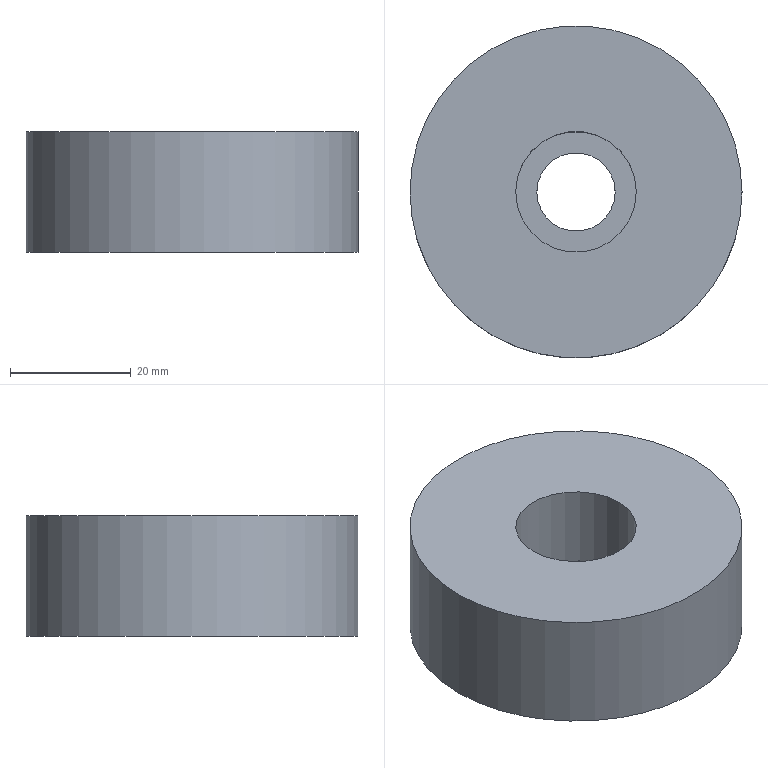Part | NX | features solid 2 | 1 solid | 6 faces | box 55 x 55 x 20 mm | volume 42322 mm3 | cylinder 3 | plane 3 | commonest cylinder face diameters 13 x1 20 x1 55 x1
STEP:
#1=CARTESIAN_POINT('',(512.5,735.,223.2));
#2=VERTEX_POINT('',#1);
#3=CARTESIAN_POINT('',(540.,735.,223.2));
#4=DIRECTION('',(0.,0.,-1.));
#5=DIRECTION('',(-1.,0.,0.));
#6=AXIS2_PLACEMENT_3D('',#3,#4,#5);
#7=CIRCLE('',#6,27.5);
#8=EDGE_CURVE('',#2,#2,#7,.T.);
#9=ORIENTED_EDGE('',*,*,#8,.T.);
#10=EDGE_LOOP('',(#9));
#11=FACE_BOUND('',#10,.T.);
#12=CARTESIAN_POINT('',(512.5,735.,203.2));
#13=VERTEX_POINT('',#12);
#14=CARTESIAN_POINT('',(540.,735.,203.2));
#15=DIRECTION('',(0.,0.,-1.));
#16=DIRECTION('',(-1.,0.,0.));
#17=AXIS2_PLACEMENT_3D('',#14,#15,#16);
#18=CIRCLE('',#17,27.5);
#19=EDGE_CURVE('',#13,#13,#18,.T.);
#20=ORIENTED_EDGE('',*,*,#19,.F.);
#21=EDGE_LOOP('',(#20));
#22=FACE_BOUND('',#21,.T.);
#23=CARTESIAN_POINT('',(540.,735.,223.2));
#24=DIRECTION('',(0.,0.,-1.));
#25=DIRECTION('',(1.,0.,0.));
#26=AXIS2_PLACEMENT_3D('',#23,#24,#25);
#27=CYLINDRICAL_SURFACE('',#26,27.5);
#28=ADVANCED_FACE('',(#11,#22),#27,.T.);
#29=CARTESIAN_POINT('',(550.,735.,223.2));
#30=VERTEX_POINT('',#29);
#31=CARTESIAN_POINT('',(540.,735.,223.2));
#32=DIRECTION('',(0.,0.,1.));
#33=DIRECTION('',(1.,0.,0.));
#34=AXIS2_PLACEMENT_3D('',#31,#32,#33);
#35=CIRCLE('',#34,10.);
#36=EDGE_CURVE('',#30,#30,#35,.T.);
#37=ORIENTED_EDGE('',*,*,#36,.F.);
#38=EDGE_LOOP('',(#37));
#39=FACE_BOUND('',#38,.T.);
#40=ORIENTED_EDGE('',*,*,#8,.F.);
#41=EDGE_LOOP('',(#40));
#42=FACE_BOUND('',#41,.T.);
#43=CARTESIAN_POINT('',(540.,735.,223.2));
#44=DIRECTION('',(0.,0.,1.));
#45=DIRECTION('',(-1.,0.,0.));
#46=AXIS2_PLACEMENT_3D('',#43,#44,#45);
#47=PLANE('',#46);
#48=ADVANCED_FACE('',(#39,#42),#47,.T.);
#49=CARTESIAN_POINT('',(533.5,735.,203.2));
#50=VERTEX_POINT('',#49);
#51=CARTESIAN_POINT('',(540.,735.,203.2));
#52=DIRECTION('',(0.,0.,-1.));
#53=DIRECTION('',(-1.,0.,0.));
#54=AXIS2_PLACEMENT_3D('',#51,#52,#53);
#55=CIRCLE('',#54,6.5);
#56=EDGE_CURVE('',#50,#50,#55,.T.);
#57=ORIENTED_EDGE('',*,*,#56,.F.);
#58=EDGE_LOOP('',(#57));
#59=FACE_BOUND('',#58,.T.);
#60=ORIENTED_EDGE('',*,*,#19,.T.);
#61=EDGE_LOOP('',(#60));
#62=FACE_BOUND('',#61,.T.);
#63=CARTESIAN_POINT('',(540.,735.,203.2));
#64=DIRECTION('',(0.,0.,1.));
#65=DIRECTION('',(-1.,0.,0.));
#66=AXIS2_PLACEMENT_3D('',#63,#64,#65);
#67=PLANE('',#66);
#68=ADVANCED_FACE('',(#59,#62),#67,.F.);
#69=CARTESIAN_POINT('',(546.5,735.,209.2));
#70=VERTEX_POINT('',#69);
#71=CARTESIAN_POINT('',(540.,735.,209.2));
#72=DIRECTION('',(0.,0.,1.));
#73=DIRECTION('',(1.,0.,0.));
#74=AXIS2_PLACEMENT_3D('',#71,#72,#73);
#75=CIRCLE('',#74,6.5);
#76=EDGE_CURVE('',#70,#70,#75,.T.);
#77=ORIENTED_EDGE('',*,*,#76,.T.);
#78=EDGE_LOOP('',(#77));
#79=FACE_BOUND('',#78,.T.);
#80=ORIENTED_EDGE('',*,*,#56,.T.);
#81=EDGE_LOOP('',(#80));
#82=FACE_BOUND('',#81,.T.);
#83=CARTESIAN_POINT('',(540.,735.,123.2));
#84=DIRECTION('',(0.,0.,-1.));
#85=DIRECTION('',(1.,0.,0.));
#86=AXIS2_PLACEMENT_3D('',#83,#84,#85);
#87=CYLINDRICAL_SURFACE('',#86,6.5);
#88=ADVANCED_FACE('',(#79,#82),#87,.F.);
#89=ORIENTED_EDGE('',*,*,#76,.F.);
#90=EDGE_LOOP('',(#89));
#91=FACE_BOUND('',#90,.T.);
#92=CARTESIAN_POINT('',(550.,735.,209.2));
#93=VERTEX_POINT('',#92);
#94=CARTESIAN_POINT('',(540.,735.,209.2));
#95=DIRECTION('',(0.,0.,1.));
#96=DIRECTION('',(1.,0.,0.));
#97=AXIS2_PLACEMENT_3D('',#94,#95,#96);
#98=CIRCLE('',#97,10.);
#99=EDGE_CURVE('',#93,#93,#98,.T.);
#100=ORIENTED_EDGE('',*,*,#99,.T.);
#101=EDGE_LOOP('',(#100));
#102=FACE_BOUND('',#101,.T.);
#103=CARTESIAN_POINT('',(540.,735.,209.2));
#104=DIRECTION('',(0.,0.,-1.));
#105=DIRECTION('',(1.,0.,0.));
#106=AXIS2_PLACEMENT_3D('',#103,#104,#105);
#107=PLANE('',#106);
#108=ADVANCED_FACE('',(#91,#102),#107,.F.);
#109=ORIENTED_EDGE('',*,*,#99,.F.);
#110=EDGE_LOOP('',(#109));
#111=FACE_BOUND('',#110,.T.);
#112=ORIENTED_EDGE('',*,*,#36,.T.);
#113=EDGE_LOOP('',(#112));
#114=FACE_BOUND('',#113,.T.);
#115=CARTESIAN_POINT('',(540.,735.,223.2));
#116=DIRECTION('',(0.,0.,-1.));
#117=DIRECTION('',(1.,0.,0.));
#118=AXIS2_PLACEMENT_3D('',#115,#116,#117);
#119=CYLINDRICAL_SURFACE('',#118,10.);
#120=ADVANCED_FACE('',(#111,#114),#119,.F.);
#121=CLOSED_SHELL('',(#28,#48,#68,#88,#108,#120));
#122=MANIFOLD_SOLID_BREP('',#121);
#123=(LENGTH_UNIT()NAMED_UNIT(*)SI_UNIT(.MILLI.,.METRE.));
#124=UNCERTAINTY_MEASURE_WITH_UNIT(LENGTH_MEASURE(0.00001),#123,'','');
#125=(NAMED_UNIT(*)PLANE_ANGLE_UNIT()SI_UNIT($,.RADIAN.));
#126=(NAMED_UNIT(*)SI_UNIT($,.STERADIAN.)SOLID_ANGLE_UNIT());
#127=(GEOMETRIC_REPRESENTATION_CONTEXT(3)GLOBAL_UNCERTAINTY_ASSIGNED_CONTEXT((#124))GLOBAL_UNIT_ASSIGNED_CONTEXT((#123,#125,#126))REPRESENTATION_CONTEXT('',''));
#128=ADVANCED_BREP_SHAPE_REPRESENTATION('',(#122),#127);